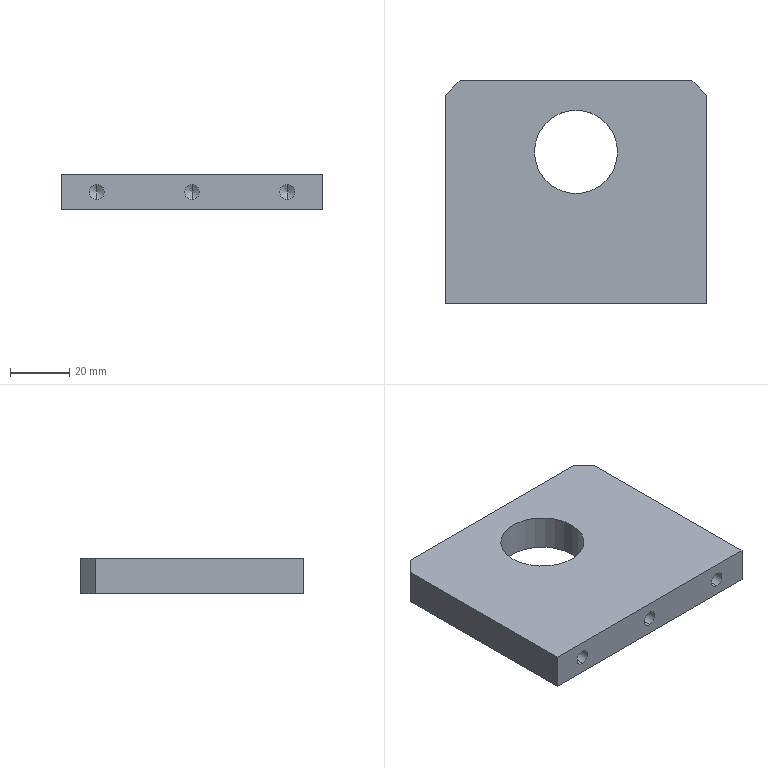Part | STEP file | mounting fixed plate | 1 solid | 22 faces | box 88 x 75 x 12 mm | volume 70480 mm3 | cylinder 8 | plane 8 | cone 6 | commonest cylinder face diameters 5 x6 28 x2
STEP:
#1=CARTESIAN_POINT('',(0.,0.,0.));
#2=DIRECTION('',(0.,0.,1.));
#3=DIRECTION('',(1.,0.,0.));
#4=AXIS2_PLACEMENT_3D('',#1,#2,#3);
#5=CARTESIAN_POINT('',(-14.,13.5,12.));
#6=VERTEX_POINT('',#5);
#7=CARTESIAN_POINT('',(-14.,13.5,0.));
#8=VERTEX_POINT('',#7);
#9=CARTESIAN_POINT('',(-14.,13.5,12.));
#10=DIRECTION('',(0.,0.,-1.));
#11=VECTOR('',#10,1.);
#12=LINE('',#9,#11);
#13=CARTESIAN_POINT('',(0.,13.5,12.));
#14=DIRECTION('',(0.,0.,-1.));
#15=DIRECTION('',(-1.,0.,0.));
#16=AXIS2_PLACEMENT_3D('',#13,#14,#15);
#17=CYLINDRICAL_SURFACE('',#16,14.);
#18=CARTESIAN_POINT('',(6.283,0.));
#19=DIRECTION('',(0.,1.));
#20=VECTOR('',#19,1.);
#21=LINE('',#18,#20);
#22=(GEOMETRIC_REPRESENTATION_CONTEXT(2)PARAMETRIC_REPRESENTATION_CONTEXT()REPRESENTATION_CONTEXT('',''));
#23=DEFINITIONAL_REPRESENTATION('',(#21),#22);
#24=PCURVE('',#17,#23);
#25=CARTESIAN_POINT('',(0.,13.5,12.));
#26=DIRECTION('',(0.,0.,-1.));
#27=DIRECTION('',(-1.,0.,0.));
#28=AXIS2_PLACEMENT_3D('',#25,#26,#27);
#29=CYLINDRICAL_SURFACE('',#28,14.);
#30=CARTESIAN_POINT('',(0.,0.));
#31=DIRECTION('',(0.,1.));
#32=VECTOR('',#31,1.);
#33=LINE('',#30,#32);
#34=(GEOMETRIC_REPRESENTATION_CONTEXT(2)PARAMETRIC_REPRESENTATION_CONTEXT()REPRESENTATION_CONTEXT('',''));
#35=DEFINITIONAL_REPRESENTATION('',(#33),#34);
#36=PCURVE('',#29,#35);
#37=SURFACE_CURVE('',#12,(#24,#36),.PCURVE_S1.);
#38=EDGE_CURVE('',#6,#8,#37,.T.);
#39=ORIENTED_EDGE('',*,*,#38,.T.);
#40=CARTESIAN_POINT('',(14.,13.5,0.));
#41=VERTEX_POINT('',#40);
#42=CARTESIAN_POINT('',(0.,13.5,0.));
#43=DIRECTION('',(0.,0.,1.));
#44=DIRECTION('',(-1.,0.,0.));
#45=AXIS2_PLACEMENT_3D('',#42,#43,#44);
#46=CIRCLE('',#45,14.);
#47=CARTESIAN_POINT('',(6.283,12.));
#48=DIRECTION('',(-1.,0.));
#49=VECTOR('',#48,1.);
#50=LINE('',#47,#49);
#51=(GEOMETRIC_REPRESENTATION_CONTEXT(2)PARAMETRIC_REPRESENTATION_CONTEXT()REPRESENTATION_CONTEXT('',''));
#52=DEFINITIONAL_REPRESENTATION('',(#50),#51);
#53=PCURVE('',#17,#52);
#54=CARTESIAN_POINT('',(-44.,37.5,0.));
#55=DIRECTION('',(0.,0.,-1.));
#56=DIRECTION('',(-1.,0.,0.));
#57=AXIS2_PLACEMENT_3D('',#54,#55,#56);
#58=PLANE('',#57);
#59=CARTESIAN_POINT('',(-30.,-24.));
#60=CARTESIAN_POINT('',(-30.,-48.249));
#61=CARTESIAN_POINT('',(-51.,-36.124));
#62=CARTESIAN_POINT('',(-72.,-24.));
#63=CARTESIAN_POINT('',(-51.,-11.876));
#64=CARTESIAN_POINT('',(-30.,0.2487));
#65=CARTESIAN_POINT('',(-30.,-24.));
#66=(BOUNDED_CURVE()B_SPLINE_CURVE(2,(#59,#60,#61,#62,#63,#64,#65),.UNSPECIFIED.,.T.,.F.)B_SPLINE_CURVE_WITH_KNOTS((1,2,2,2,2,1),(-2.094,0.,2.094,4.189,6.283,8.378),.UNSPECIFIED.)CURVE()GEOMETRIC_REPRESENTATION_ITEM()RATIONAL_B_SPLINE_CURVE((1.,0.5,1.,0.5,1.,0.5,1.))REPRESENTATION_ITEM(''));
#67=(GEOMETRIC_REPRESENTATION_CONTEXT(2)PARAMETRIC_REPRESENTATION_CONTEXT()REPRESENTATION_CONTEXT('',''));
#68=DEFINITIONAL_REPRESENTATION('',(#66),#67);
#69=PCURVE('',#58,#68);
#70=SURFACE_CURVE('',#46,(#53,#69),.PCURVE_S1.);
#71=EDGE_CURVE('',#8,#41,#70,.T.);
#72=ORIENTED_EDGE('',*,*,#71,.T.);
#73=CARTESIAN_POINT('',(14.,13.5,12.));
#74=VERTEX_POINT('',#73);
#75=CARTESIAN_POINT('',(14.,13.5,12.));
#76=DIRECTION('',(0.,0.,-1.));
#77=VECTOR('',#76,1.);
#78=LINE('',#75,#77);
#79=CARTESIAN_POINT('',(3.142,0.));
#80=DIRECTION('',(0.,1.));
#81=VECTOR('',#80,1.);
#82=LINE('',#79,#81);
#83=(GEOMETRIC_REPRESENTATION_CONTEXT(2)PARAMETRIC_REPRESENTATION_CONTEXT()REPRESENTATION_CONTEXT('',''));
#84=DEFINITIONAL_REPRESENTATION('',(#82),#83);
#85=PCURVE('',#17,#84);
#86=CARTESIAN_POINT('',(3.142,0.));
#87=DIRECTION('',(0.,1.));
#88=VECTOR('',#87,1.);
#89=LINE('',#86,#88);
#90=(GEOMETRIC_REPRESENTATION_CONTEXT(2)PARAMETRIC_REPRESENTATION_CONTEXT()REPRESENTATION_CONTEXT('',''));
#91=DEFINITIONAL_REPRESENTATION('',(#89),#90);
#92=PCURVE('',#29,#91);
#93=SURFACE_CURVE('',#78,(#85,#92),.PCURVE_S1.);
#94=EDGE_CURVE('',#74,#41,#93,.T.);
#95=ORIENTED_EDGE('',*,*,#94,.F.);
#96=CARTESIAN_POINT('',(0.,13.5,12.));
#97=DIRECTION('',(0.,0.,1.));
#98=DIRECTION('',(-1.,0.,0.));
#99=AXIS2_PLACEMENT_3D('',#96,#97,#98);
#100=CIRCLE('',#99,14.);
#101=CARTESIAN_POINT('',(6.283,0.));
#102=DIRECTION('',(-1.,0.));
#103=VECTOR('',#102,1.);
#104=LINE('',#101,#103);
#105=(GEOMETRIC_REPRESENTATION_CONTEXT(2)PARAMETRIC_REPRESENTATION_CONTEXT()REPRESENTATION_CONTEXT('',''));
#106=DEFINITIONAL_REPRESENTATION('',(#104),#105);
#107=PCURVE('',#17,#106);
#108=CARTESIAN_POINT('',(-44.,37.5,12.));
#109=DIRECTION('',(0.,0.,-1.));
#110=DIRECTION('',(-1.,0.,0.));
#111=AXIS2_PLACEMENT_3D('',#108,#109,#110);
#112=PLANE('',#111);
#113=CARTESIAN_POINT('',(-30.,-24.));
#114=CARTESIAN_POINT('',(-30.,-48.249));
#115=CARTESIAN_POINT('',(-51.,-36.124));
#116=CARTESIAN_POINT('',(-72.,-24.));
#117=CARTESIAN_POINT('',(-51.,-11.876));
#118=CARTESIAN_POINT('',(-30.,0.2487));
#119=CARTESIAN_POINT('',(-30.,-24.));
#120=(BOUNDED_CURVE()B_SPLINE_CURVE(2,(#113,#114,#115,#116,#117,#118,#119),.UNSPECIFIED.,.T.,.F.)B_SPLINE_CURVE_WITH_KNOTS((1,2,2,2,2,1),(-2.094,0.,2.094,4.189,6.283,8.378),.UNSPECIFIED.)CURVE()GEOMETRIC_REPRESENTATION_ITEM()RATIONAL_B_SPLINE_CURVE((1.,0.5,1.,0.5,1.,0.5,1.))REPRESENTATION_ITEM(''));
#121=(GEOMETRIC_REPRESENTATION_CONTEXT(2)PARAMETRIC_REPRESENTATION_CONTEXT()REPRESENTATION_CONTEXT('',''));
#122=DEFINITIONAL_REPRESENTATION('',(#120),#121);
#123=PCURVE('',#112,#122);
#124=SURFACE_CURVE('',#100,(#107,#123),.PCURVE_S1.);
#125=EDGE_CURVE('',#6,#74,#124,.T.);
#126=ORIENTED_EDGE('',*,*,#125,.F.);
#127=EDGE_LOOP('',(#39,#72,#95,#126));
#128=FACE_BOUND('',#127,.F.);
#129=ADVANCED_FACE('',(#128),#17,.F.);
#130=CARTESIAN_POINT('',(-32.,-20.5,3.5));
#131=VERTEX_POINT('',#130);
#132=CARTESIAN_POINT('',(-32.,-37.5,3.5));
#133=VERTEX_POINT('',#132);
#134=CARTESIAN_POINT('',(-32.,-37.5,3.5));
#135=DIRECTION('',(0.,-1.,0.));
#136=VECTOR('',#135,1.);
#137=LINE('',#134,#136);
#138=CARTESIAN_POINT('',(-32.,-37.5,6.));
#139=DIRECTION('',(0.,-1.,0.));
#140=DIRECTION('',(0.,0.,-1.));
#141=AXIS2_PLACEMENT_3D('',#138,#139,#140);
#142=CYLINDRICAL_SURFACE('',#141,2.5);
#143=CARTESIAN_POINT('',(6.283,0.));
#144=DIRECTION('',(0.,1.));
#145=VECTOR('',#144,1.);
#146=LINE('',#143,#145);
#147=(GEOMETRIC_REPRESENTATION_CONTEXT(2)PARAMETRIC_REPRESENTATION_CONTEXT()REPRESENTATION_CONTEXT('',''));
#148=DEFINITIONAL_REPRESENTATION('',(#146),#147);
#149=PCURVE('',#142,#148);
#150=CARTESIAN_POINT('',(-32.,-37.5,6.));
#151=DIRECTION('',(0.,-1.,0.));
#152=DIRECTION('',(0.,0.,-1.));
#153=AXIS2_PLACEMENT_3D('',#150,#151,#152);
#154=CYLINDRICAL_SURFACE('',#153,2.5);
#155=CARTESIAN_POINT('',(0.,0.));
#156=DIRECTION('',(0.,1.));
#157=VECTOR('',#156,1.);
#158=LINE('',#155,#157);
#159=(GEOMETRIC_REPRESENTATION_CONTEXT(2)PARAMETRIC_REPRESENTATION_CONTEXT()REPRESENTATION_CONTEXT('',''));
#160=DEFINITIONAL_REPRESENTATION('',(#158),#159);
#161=PCURVE('',#154,#160);
#162=SURFACE_CURVE('',#137,(#149,#161),.PCURVE_S1.);
#163=EDGE_CURVE('',#131,#133,#162,.T.);
#164=ORIENTED_EDGE('',*,*,#163,.T.);
#165=CARTESIAN_POINT('',(-32.,-37.5,8.5));
#166=VERTEX_POINT('',#165);
#167=CARTESIAN_POINT('',(-32.,-37.5,6.));
#168=DIRECTION('',(0.,-1.,0.));
#169=DIRECTION('',(0.,0.,-1.));
#170=AXIS2_PLACEMENT_3D('',#167,#168,#169);
#171=CIRCLE('',#170,2.5);
#172=CARTESIAN_POINT('',(0.,0.));
#173=DIRECTION('',(1.,0.));
#174=VECTOR('',#173,1.);
#175=LINE('',#172,#174);
#176=(GEOMETRIC_REPRESENTATION_CONTEXT(2)PARAMETRIC_REPRESENTATION_CONTEXT()REPRESENTATION_CONTEXT('',''));
#177=DEFINITIONAL_REPRESENTATION('',(#175),#176);
#178=PCURVE('',#142,#177);
#179=CARTESIAN_POINT('',(-44.,-37.5,12.));
#180=DIRECTION('',(0.,1.,0.));
#181=DIRECTION('',(0.,0.,1.));
#182=AXIS2_PLACEMENT_3D('',#179,#180,#181);
#183=PLANE('',#182);
#184=CARTESIAN_POINT('',(-8.5,12.));
#185=CARTESIAN_POINT('',(-8.5,16.33));
#186=CARTESIAN_POINT('',(-4.75,14.165));
#187=CARTESIAN_POINT('',(-1.,12.));
#188=CARTESIAN_POINT('',(-4.75,9.835));
#189=CARTESIAN_POINT('',(-8.5,7.67));
#190=CARTESIAN_POINT('',(-8.5,12.));
#191=(BOUNDED_CURVE()B_SPLINE_CURVE(2,(#184,#185,#186,#187,#188,#189,#190),.UNSPECIFIED.,.T.,.F.)B_SPLINE_CURVE_WITH_KNOTS((1,2,2,2,2,1),(-2.094,0.,2.094,4.189,6.283,8.378),.UNSPECIFIED.)CURVE()GEOMETRIC_REPRESENTATION_ITEM()RATIONAL_B_SPLINE_CURVE((1.,0.5,1.,0.5,1.,0.5,1.))REPRESENTATION_ITEM(''));
#192=(GEOMETRIC_REPRESENTATION_CONTEXT(2)PARAMETRIC_REPRESENTATION_CONTEXT()REPRESENTATION_CONTEXT('',''));
#193=DEFINITIONAL_REPRESENTATION('',(#191),#192);
#194=PCURVE('',#183,#193);
#195=SURFACE_CURVE('',#171,(#178,#194),.PCURVE_S1.);
#196=EDGE_CURVE('',#166,#133,#195,.T.);
#197=ORIENTED_EDGE('',*,*,#196,.F.);
#198=CARTESIAN_POINT('',(-32.,-20.5,8.5));
#199=VERTEX_POINT('',#198);
#200=CARTESIAN_POINT('',(-32.,-37.5,8.5));
#201=DIRECTION('',(0.,-1.,0.));
#202=VECTOR('',#201,1.);
#203=LINE('',#200,#202);
#204=CARTESIAN_POINT('',(3.142,0.));
#205=DIRECTION('',(0.,1.));
#206=VECTOR('',#205,1.);
#207=LINE('',#204,#206);
#208=(GEOMETRIC_REPRESENTATION_CONTEXT(2)PARAMETRIC_REPRESENTATION_CONTEXT()REPRESENTATION_CONTEXT('',''));
#209=DEFINITIONAL_REPRESENTATION('',(#207),#208);
#210=PCURVE('',#142,#209);
#211=CARTESIAN_POINT('',(3.142,0.));
#212=DIRECTION('',(0.,1.));
#213=VECTOR('',#212,1.);
#214=LINE('',#211,#213);
#215=(GEOMETRIC_REPRESENTATION_CONTEXT(2)PARAMETRIC_REPRESENTATION_CONTEXT()REPRESENTATION_CONTEXT('',''));
#216=DEFINITIONAL_REPRESENTATION('',(#214),#215);
#217=PCURVE('',#154,#216);
#218=SURFACE_CURVE('',#203,(#210,#217),.PCURVE_S1.);
#219=EDGE_CURVE('',#199,#166,#218,.T.);
#220=ORIENTED_EDGE('',*,*,#219,.F.);
#221=CARTESIAN_POINT('',(-32.,-20.5,6.));
#222=DIRECTION('',(0.,-1.,0.));
#223=DIRECTION('',(0.,0.,-1.));
#224=AXIS2_PLACEMENT_3D('',#221,#222,#223);
#225=CIRCLE('',#224,2.5);
#226=CARTESIAN_POINT('',(0.,-17.));
#227=DIRECTION('',(1.,0.));
#228=VECTOR('',#227,1.);
#229=LINE('',#226,#228);
#230=(GEOMETRIC_REPRESENTATION_CONTEXT(2)PARAMETRIC_REPRESENTATION_CONTEXT()REPRESENTATION_CONTEXT('',''));
#231=DEFINITIONAL_REPRESENTATION('',(#229),#230);
#232=PCURVE('',#142,#231);
#233=CARTESIAN_POINT('',(-32.,-20.5,6.));
#234=DIRECTION('',(0.,-1.,0.));
#235=DIRECTION('',(0.,0.,-1.));
#236=AXIS2_PLACEMENT_3D('',#233,#234,#235);
#237=CONICAL_SURFACE('',#236,2.5,1.03);
#238=CARTESIAN_POINT('',(0.,0.));
#239=DIRECTION('',(1.,0.));
#240=VECTOR('',#239,1.);
#241=LINE('',#238,#240);
#242=(GEOMETRIC_REPRESENTATION_CONTEXT(2)PARAMETRIC_REPRESENTATION_CONTEXT()REPRESENTATION_CONTEXT('',''));
#243=DEFINITIONAL_REPRESENTATION('',(#241),#242);
#244=PCURVE('',#237,#243);
#245=SURFACE_CURVE('',#225,(#232,#244),.PCURVE_S1.);
#246=EDGE_CURVE('',#199,#131,#245,.T.);
#247=ORIENTED_EDGE('',*,*,#246,.T.);
#248=EDGE_LOOP('',(#164,#197,#220,#247));
#249=FACE_BOUND('',#248,.F.);
#250=ADVANCED_FACE('',(#249),#142,.F.);
#251=CARTESIAN_POINT('',(32.,-20.5,3.5));
#252=VERTEX_POINT('',#251);
#253=CARTESIAN_POINT('',(32.,-37.5,3.5));
#254=VERTEX_POINT('',#253);
#255=CARTESIAN_POINT('',(32.,-37.5,3.5));
#256=DIRECTION('',(0.,-1.,0.));
#257=VECTOR('',#256,1.);
#258=LINE('',#255,#257);
#259=CARTESIAN_POINT('',(32.,-37.5,6.));
#260=DIRECTION('',(0.,-1.,0.));
#261=DIRECTION('',(0.,0.,-1.));
#262=AXIS2_PLACEMENT_3D('',#259,#260,#261);
#263=CYLINDRICAL_SURFACE('',#262,2.5);
#264=CARTESIAN_POINT('',(6.283,0.));
#265=DIRECTION('',(0.,1.));
#266=VECTOR('',#265,1.);
#267=LINE('',#264,#266);
#268=(GEOMETRIC_REPRESENTATION_CONTEXT(2)PARAMETRIC_REPRESENTATION_CONTEXT()REPRESENTATION_CONTEXT('',''));
#269=DEFINITIONAL_REPRESENTATION('',(#267),#268);
#270=PCURVE('',#263,#269);
#271=CARTESIAN_POINT('',(32.,-37.5,6.));
#272=DIRECTION('',(0.,-1.,0.));
#273=DIRECTION('',(0.,0.,-1.));
#274=AXIS2_PLACEMENT_3D('',#271,#272,#273);
#275=CYLINDRICAL_SURFACE('',#274,2.5);
#276=CARTESIAN_POINT('',(0.,0.));
#277=DIRECTION('',(0.,1.));
#278=VECTOR('',#277,1.);
#279=LINE('',#276,#278);
#280=(GEOMETRIC_REPRESENTATION_CONTEXT(2)PARAMETRIC_REPRESENTATION_CONTEXT()REPRESENTATION_CONTEXT('',''));
#281=DEFINITIONAL_REPRESENTATION('',(#279),#280);
#282=PCURVE('',#275,#281);
#283=SURFACE_CURVE('',#258,(#270,#282),.PCURVE_S1.);
#284=EDGE_CURVE('',#252,#254,#283,.T.);
#285=ORIENTED_EDGE('',*,*,#284,.T.);
#286=CARTESIAN_POINT('',(32.,-37.5,8.5));
#287=VERTEX_POINT('',#286);
#288=CARTESIAN_POINT('',(32.,-37.5,6.));
#289=DIRECTION('',(0.,-1.,0.));
#290=DIRECTION('',(0.,0.,-1.));
#291=AXIS2_PLACEMENT_3D('',#288,#289,#290);
#292=CIRCLE('',#291,2.5);
#293=CARTESIAN_POINT('',(0.,0.));
#294=DIRECTION('',(1.,0.));
#295=VECTOR('',#294,1.);
#296=LINE('',#293,#295);
#297=(GEOMETRIC_REPRESENTATION_CONTEXT(2)PARAMETRIC_REPRESENTATION_CONTEXT()REPRESENTATION_CONTEXT('',''));
#298=DEFINITIONAL_REPRESENTATION('',(#296),#297);
#299=PCURVE('',#263,#298);
#300=CARTESIAN_POINT('',(-8.5,76.));
#301=CARTESIAN_POINT('',(-8.5,80.33));
#302=CARTESIAN_POINT('',(-4.75,78.165));
#303=CARTESIAN_POINT('',(-1.,76.));
#304=CARTESIAN_POINT('',(-4.75,73.835));
#305=CARTESIAN_POINT('',(-8.5,71.67));
#306=CARTESIAN_POINT('',(-8.5,76.));
#307=(BOUNDED_CURVE()B_SPLINE_CURVE(2,(#300,#301,#302,#303,#304,#305,#306),.UNSPECIFIED.,.T.,.F.)B_SPLINE_CURVE_WITH_KNOTS((1,2,2,2,2,1),(-2.094,0.,2.094,4.189,6.283,8.378),.UNSPECIFIED.)CURVE()GEOMETRIC_REPRESENTATION_ITEM()RATIONAL_B_SPLINE_CURVE((1.,0.5,1.,0.5,1.,0.5,1.))REPRESENTATION_ITEM(''));
#308=(GEOMETRIC_REPRESENTATION_CONTEXT(2)PARAMETRIC_REPRESENTATION_CONTEXT()REPRESENTATION_CONTEXT('',''));
#309=DEFINITIONAL_REPRESENTATION('',(#307),#308);
#310=PCURVE('',#183,#309);
#311=SURFACE_CURVE('',#292,(#299,#310),.PCURVE_S1.);
#312=EDGE_CURVE('',#287,#254,#311,.T.);
#313=ORIENTED_EDGE('',*,*,#312,.F.);
#314=CARTESIAN_POINT('',(32.,-20.5,8.5));
#315=VERTEX_POINT('',#314);
#316=CARTESIAN_POINT('',(32.,-37.5,8.5));
#317=DIRECTION('',(0.,-1.,0.));
#318=VECTOR('',#317,1.);
#319=LINE('',#316,#318);
#320=CARTESIAN_POINT('',(3.142,0.));
#321=DIRECTION('',(0.,1.));
#322=VECTOR('',#321,1.);
#323=LINE('',#320,#322);
#324=(GEOMETRIC_REPRESENTATION_CONTEXT(2)PARAMETRIC_REPRESENTATION_CONTEXT()REPRESENTATION_CONTEXT('',''));
#325=DEFINITIONAL_REPRESENTATION('',(#323),#324);
#326=PCURVE('',#263,#325);
#327=CARTESIAN_POINT('',(3.142,0.));
#328=DIRECTION('',(0.,1.));
#329=VECTOR('',#328,1.);
#330=LINE('',#327,#329);
#331=(GEOMETRIC_REPRESENTATION_CONTEXT(2)PARAMETRIC_REPRESENTATION_CONTEXT()REPRESENTATION_CONTEXT('',''));
#332=DEFINITIONAL_REPRESENTATION('',(#330),#331);
#333=PCURVE('',#275,#332);
#334=SURFACE_CURVE('',#319,(#326,#333),.PCURVE_S1.);
#335=EDGE_CURVE('',#315,#287,#334,.T.);
#336=ORIENTED_EDGE('',*,*,#335,.F.);
#337=CARTESIAN_POINT('',(32.,-20.5,6.));
#338=DIRECTION('',(0.,-1.,0.));
#339=DIRECTION('',(0.,0.,-1.));
#340=AXIS2_PLACEMENT_3D('',#337,#338,#339);
#341=CIRCLE('',#340,2.5);
#342=CARTESIAN_POINT('',(0.,-17.));
#343=DIRECTION('',(1.,0.));
#344=VECTOR('',#343,1.);
#345=LINE('',#342,#344);
#346=(GEOMETRIC_REPRESENTATION_CONTEXT(2)PARAMETRIC_REPRESENTATION_CONTEXT()REPRESENTATION_CONTEXT('',''));
#347=DEFINITIONAL_REPRESENTATION('',(#345),#346);
#348=PCURVE('',#263,#347);
#349=CARTESIAN_POINT('',(32.,-20.5,6.));
#350=DIRECTION('',(0.,-1.,0.));
#351=DIRECTION('',(0.,0.,-1.));
#352=AXIS2_PLACEMENT_3D('',#349,#350,#351);
#353=CONICAL_SURFACE('',#352,2.5,1.03);
#354=CARTESIAN_POINT('',(0.,0.));
#355=DIRECTION('',(1.,0.));
#356=VECTOR('',#355,1.);
#357=LINE('',#354,#356);
#358=(GEOMETRIC_REPRESENTATION_CONTEXT(2)PARAMETRIC_REPRESENTATION_CONTEXT()REPRESENTATION_CONTEXT('',''));
#359=DEFINITIONAL_REPRESENTATION('',(#357),#358);
#360=PCURVE('',#353,#359);
#361=SURFACE_CURVE('',#341,(#348,#360),.PCURVE_S1.);
#362=EDGE_CURVE('',#315,#252,#361,.T.);
#363=ORIENTED_EDGE('',*,*,#362,.T.);
#364=EDGE_LOOP('',(#285,#313,#336,#363));
#365=FACE_BOUND('',#364,.F.);
#366=ADVANCED_FACE('',(#365),#263,.F.);
#367=CARTESIAN_POINT('',(0.,-20.5,3.5));
#368=VERTEX_POINT('',#367);
#369=CARTESIAN_POINT('',(0.,-37.5,3.5));
#370=VERTEX_POINT('',#369);
#371=CARTESIAN_POINT('',(0.,-37.5,3.5));
#372=DIRECTION('',(0.,-1.,0.));
#373=VECTOR('',#372,1.);
#374=LINE('',#371,#373);
#375=CARTESIAN_POINT('',(0.,-37.5,6.));
#376=DIRECTION('',(0.,-1.,0.));
#377=DIRECTION('',(0.,0.,-1.));
#378=AXIS2_PLACEMENT_3D('',#375,#376,#377);
#379=CYLINDRICAL_SURFACE('',#378,2.5);
#380=CARTESIAN_POINT('',(6.283,0.));
#381=DIRECTION('',(0.,1.));
#382=VECTOR('',#381,1.);
#383=LINE('',#380,#382);
#384=(GEOMETRIC_REPRESENTATION_CONTEXT(2)PARAMETRIC_REPRESENTATION_CONTEXT()REPRESENTATION_CONTEXT('',''));
#385=DEFINITIONAL_REPRESENTATION('',(#383),#384);
#386=PCURVE('',#379,#385);
#387=CARTESIAN_POINT('',(0.,-37.5,6.));
#388=DIRECTION('',(0.,-1.,0.));
#389=DIRECTION('',(0.,0.,-1.));
#390=AXIS2_PLACEMENT_3D('',#387,#388,#389);
#391=CYLINDRICAL_SURFACE('',#390,2.5);
#392=CARTESIAN_POINT('',(0.,0.));
#393=DIRECTION('',(0.,1.));
#394=VECTOR('',#393,1.);
#395=LINE('',#392,#394);
#396=(GEOMETRIC_REPRESENTATION_CONTEXT(2)PARAMETRIC_REPRESENTATION_CONTEXT()REPRESENTATION_CONTEXT('',''));
#397=DEFINITIONAL_REPRESENTATION('',(#395),#396);
#398=PCURVE('',#391,#397);
#399=SURFACE_CURVE('',#374,(#386,#398),.PCURVE_S1.);
#400=EDGE_CURVE('',#368,#370,#399,.T.);
#401=ORIENTED_EDGE('',*,*,#400,.T.);
#402=CARTESIAN_POINT('',(0.,-37.5,8.5));
#403=VERTEX_POINT('',#402);
#404=CARTESIAN_POINT('',(0.,-37.5,6.));
#405=DIRECTION('',(0.,-1.,0.));
#406=DIRECTION('',(0.,0.,-1.));
#407=AXIS2_PLACEMENT_3D('',#404,#405,#406);
#408=CIRCLE('',#407,2.5);
#409=CARTESIAN_POINT('',(0.,0.));
#410=DIRECTION('',(1.,0.));
#411=VECTOR('',#410,1.);
#412=LINE('',#409,#411);
#413=(GEOMETRIC_REPRESENTATION_CONTEXT(2)PARAMETRIC_REPRESENTATION_CONTEXT()REPRESENTATION_CONTEXT('',''));
#414=DEFINITIONAL_REPRESENTATION('',(#412),#413);
#415=PCURVE('',#379,#414);
#416=CARTESIAN_POINT('',(-8.5,44.));
#417=CARTESIAN_POINT('',(-8.5,48.33));
#418=CARTESIAN_POINT('',(-4.75,46.165));
#419=CARTESIAN_POINT('',(-1.,44.));
#420=CARTESIAN_POINT('',(-4.75,41.835));
#421=CARTESIAN_POINT('',(-8.5,39.67));
#422=CARTESIAN_POINT('',(-8.5,44.));
#423=(BOUNDED_CURVE()B_SPLINE_CURVE(2,(#416,#417,#418,#419,#420,#421,#422),.UNSPECIFIED.,.T.,.F.)B_SPLINE_CURVE_WITH_KNOTS((1,2,2,2,2,1),(-2.094,0.,2.094,4.189,6.283,8.378),.UNSPECIFIED.)CURVE()GEOMETRIC_REPRESENTATION_ITEM()RATIONAL_B_SPLINE_CURVE((1.,0.5,1.,0.5,1.,0.5,1.))REPRESENTATION_ITEM(''));
#424=(GEOMETRIC_REPRESENTATION_CONTEXT(2)PARAMETRIC_REPRESENTATION_CONTEXT()REPRESENTATION_CONTEXT('',''));
#425=DEFINITIONAL_REPRESENTATION('',(#423),#424);
#426=PCURVE('',#183,#425);
#427=SURFACE_CURVE('',#408,(#415,#426),.PCURVE_S1.);
#428=EDGE_CURVE('',#403,#370,#427,.T.);
#429=ORIENTED_EDGE('',*,*,#428,.F.);
#430=CARTESIAN_POINT('',(0.,-20.5,8.5));
#431=VERTEX_POINT('',#430);
#432=CARTESIAN_POINT('',(0.,-37.5,8.5));
#433=DIRECTION('',(0.,-1.,0.));
#434=VECTOR('',#433,1.);
#435=LINE('',#432,#434);
#436=CARTESIAN_POINT('',(3.142,0.));
#437=DIRECTION('',(0.,1.));
#438=VECTOR('',#437,1.);
#439=LINE('',#436,#438);
#440=(GEOMETRIC_REPRESENTATION_CONTEXT(2)PARAMETRIC_REPRESENTATION_CONTEXT()REPRESENTATION_CONTEXT('',''));
#441=DEFINITIONAL_REPRESENTATION('',(#439),#440);
#442=PCURVE('',#379,#441);
#443=CARTESIAN_POINT('',(3.142,0.));
#444=DIRECTION('',(0.,1.));
#445=VECTOR('',#444,1.);
#446=LINE('',#443,#445);
#447=(GEOMETRIC_REPRESENTATION_CONTEXT(2)PARAMETRIC_REPRESENTATION_CONTEXT()REPRESENTATION_CONTEXT('',''));
#448=DEFINITIONAL_REPRESENTATION('',(#446),#447);
#449=PCURVE('',#391,#448);
#450=SURFACE_CURVE('',#435,(#442,#449),.PCURVE_S1.);
#451=EDGE_CURVE('',#431,#403,#450,.T.);
#452=ORIENTED_EDGE('',*,*,#451,.F.);
#453=CARTESIAN_POINT('',(0.,-20.5,6.));
#454=DIRECTION('',(0.,-1.,0.));
#455=DIRECTION('',(0.,0.,-1.));
#456=AXIS2_PLACEMENT_3D('',#453,#454,#455);
#457=CIRCLE('',#456,2.5);
#458=CARTESIAN_POINT('',(0.,-17.));
#459=DIRECTION('',(1.,0.));
#460=VECTOR('',#459,1.);
#461=LINE('',#458,#460);
#462=(GEOMETRIC_REPRESENTATION_CONTEXT(2)PARAMETRIC_REPRESENTATION_CONTEXT()REPRESENTATION_CONTEXT('',''));
#463=DEFINITIONAL_REPRESENTATION('',(#461),#462);
#464=PCURVE('',#379,#463);
#465=CARTESIAN_POINT('',(0.,-20.5,6.));
#466=DIRECTION('',(0.,-1.,0.));
#467=DIRECTION('',(0.,0.,-1.));
#468=AXIS2_PLACEMENT_3D('',#465,#466,#467);
#469=CONICAL_SURFACE('',#468,2.5,1.03);
#470=CARTESIAN_POINT('',(0.,0.));
#471=DIRECTION('',(1.,0.));
#472=VECTOR('',#471,1.);
#473=LINE('',#470,#472);
#474=(GEOMETRIC_REPRESENTATION_CONTEXT(2)PARAMETRIC_REPRESENTATION_CONTEXT()REPRESENTATION_CONTEXT('',''));
#475=DEFINITIONAL_REPRESENTATION('',(#473),#474);
#476=PCURVE('',#469,#475);
#477=SURFACE_CURVE('',#457,(#464,#476),.PCURVE_S1.);
#478=EDGE_CURVE('',#431,#368,#477,.T.);
#479=ORIENTED_EDGE('',*,*,#478,.T.);
#480=EDGE_LOOP('',(#401,#429,#452,#479));
#481=FACE_BOUND('',#480,.F.);
#482=ADVANCED_FACE('',(#481),#379,.F.);
#483=ORIENTED_EDGE('',*,*,#246,.F.);
#484=CARTESIAN_POINT('',(-32.,-18.998,6.));
#485=VERTEX_POINT('',#484);
#486=CARTESIAN_POINT('',(-32.,-20.5,8.5));
#487=DIRECTION('',(0.,-0.515,0.8572));
#488=VECTOR('',#487,1.);
#489=LINE('',#486,#488);
#490=CARTESIAN_POINT('',(3.142,0.));
#491=DIRECTION('',(0.,1.));
#492=VECTOR('',#491,1.);
#493=LINE('',#490,#492);
#494=(GEOMETRIC_REPRESENTATION_CONTEXT(2)PARAMETRIC_REPRESENTATION_CONTEXT()REPRESENTATION_CONTEXT('',''));
#495=DEFINITIONAL_REPRESENTATION('',(#493),#494);
#496=PCURVE('',#237,#495);
#497=CARTESIAN_POINT('',(-32.,-20.5,6.));
#498=DIRECTION('',(0.,-1.,0.));
#499=DIRECTION('',(0.,0.,-1.));
#500=AXIS2_PLACEMENT_3D('',#497,#498,#499);
#501=CONICAL_SURFACE('',#500,2.5,1.03);
#502=CARTESIAN_POINT('',(3.142,0.));
#503=DIRECTION('',(0.,1.));
#504=VECTOR('',#503,1.);
#505=LINE('',#502,#504);
#506=(GEOMETRIC_REPRESENTATION_CONTEXT(2)PARAMETRIC_REPRESENTATION_CONTEXT()REPRESENTATION_CONTEXT('',''));
#507=DEFINITIONAL_REPRESENTATION('',(#505),#506);
#508=PCURVE('',#501,#507);
#509=SURFACE_CURVE('',#489,(#496,#508),.PCURVE_S1.);
#510=EDGE_CURVE('',#485,#199,#509,.T.);
#511=ORIENTED_EDGE('',*,*,#510,.F.);
#512=CARTESIAN_POINT('',(-32.,-20.5,3.5));
#513=DIRECTION('',(0.,-0.515,-0.8572));
#514=VECTOR('',#513,1.);
#515=LINE('',#512,#514);
#516=CARTESIAN_POINT('',(6.283,0.));
#517=DIRECTION('',(0.,1.));
#518=VECTOR('',#517,1.);
#519=LINE('',#516,#518);
#520=(GEOMETRIC_REPRESENTATION_CONTEXT(2)PARAMETRIC_REPRESENTATION_CONTEXT()REPRESENTATION_CONTEXT('',''));
#521=DEFINITIONAL_REPRESENTATION('',(#519),#520);
#522=PCURVE('',#237,#521);
#523=CARTESIAN_POINT('',(0.,0.));
#524=DIRECTION('',(0.,1.));
#525=VECTOR('',#524,1.);
#526=LINE('',#523,#525);
#527=(GEOMETRIC_REPRESENTATION_CONTEXT(2)PARAMETRIC_REPRESENTATION_CONTEXT()REPRESENTATION_CONTEXT('',''));
#528=DEFINITIONAL_REPRESENTATION('',(#526),#527);
#529=PCURVE('',#501,#528);
#530=SURFACE_CURVE('',#515,(#522,#529),.PCURVE_S1.);
#531=EDGE_CURVE('',#485,#131,#530,.T.);
#532=ORIENTED_EDGE('',*,*,#531,.T.);
#533=EDGE_LOOP('',(#483,#511,#532));
#534=FACE_BOUND('',#533,.F.);
#535=ADVANCED_FACE('',(#534),#237,.F.);
#536=ORIENTED_EDGE('',*,*,#362,.F.);
#537=CARTESIAN_POINT('',(32.,-18.998,6.));
#538=VERTEX_POINT('',#537);
#539=CARTESIAN_POINT('',(32.,-20.5,8.5));
#540=DIRECTION('',(0.,-0.515,0.8572));
#541=VECTOR('',#540,1.);
#542=LINE('',#539,#541);
#543=CARTESIAN_POINT('',(3.142,0.));
#544=DIRECTION('',(0.,1.));
#545=VECTOR('',#544,1.);
#546=LINE('',#543,#545);
#547=(GEOMETRIC_REPRESENTATION_CONTEXT(2)PARAMETRIC_REPRESENTATION_CONTEXT()REPRESENTATION_CONTEXT('',''));
#548=DEFINITIONAL_REPRESENTATION('',(#546),#547);
#549=PCURVE('',#353,#548);
#550=CARTESIAN_POINT('',(32.,-20.5,6.));
#551=DIRECTION('',(0.,-1.,0.));
#552=DIRECTION('',(0.,0.,-1.));
#553=AXIS2_PLACEMENT_3D('',#550,#551,#552);
#554=CONICAL_SURFACE('',#553,2.5,1.03);
#555=CARTESIAN_POINT('',(3.142,0.));
#556=DIRECTION('',(0.,1.));
#557=VECTOR('',#556,1.);
#558=LINE('',#555,#557);
#559=(GEOMETRIC_REPRESENTATION_CONTEXT(2)PARAMETRIC_REPRESENTATION_CONTEXT()REPRESENTATION_CONTEXT('',''));
#560=DEFINITIONAL_REPRESENTATION('',(#558),#559);
#561=PCURVE('',#554,#560);
#562=SURFACE_CURVE('',#542,(#549,#561),.PCURVE_S1.);
#563=EDGE_CURVE('',#538,#315,#562,.T.);
#564=ORIENTED_EDGE('',*,*,#563,.F.);
#565=CARTESIAN_POINT('',(32.,-20.5,3.5));
#566=DIRECTION('',(0.,-0.515,-0.8572));
#567=VECTOR('',#566,1.);
#568=LINE('',#565,#567);
#569=CARTESIAN_POINT('',(6.283,0.));
#570=DIRECTION('',(0.,1.));
#571=VECTOR('',#570,1.);
#572=LINE('',#569,#571);
#573=(GEOMETRIC_REPRESENTATION_CONTEXT(2)PARAMETRIC_REPRESENTATION_CONTEXT()REPRESENTATION_CONTEXT('',''));
#574=DEFINITIONAL_REPRESENTATION('',(#572),#573);
#575=PCURVE('',#353,#574);
#576=CARTESIAN_POINT('',(0.,0.));
#577=DIRECTION('',(0.,1.));
#578=VECTOR('',#577,1.);
#579=LINE('',#576,#578);
#580=(GEOMETRIC_REPRESENTATION_CONTEXT(2)PARAMETRIC_REPRESENTATION_CONTEXT()REPRESENTATION_CONTEXT('',''));
#581=DEFINITIONAL_REPRESENTATION('',(#579),#580);
#582=PCURVE('',#554,#581);
#583=SURFACE_CURVE('',#568,(#575,#582),.PCURVE_S1.);
#584=EDGE_CURVE('',#538,#252,#583,.T.);
#585=ORIENTED_EDGE('',*,*,#584,.T.);
#586=EDGE_LOOP('',(#536,#564,#585));
#587=FACE_BOUND('',#586,.F.);
#588=ADVANCED_FACE('',(#587),#353,.F.);
#589=ORIENTED_EDGE('',*,*,#478,.F.);
#590=CARTESIAN_POINT('',(0.,-18.998,6.));
#591=VERTEX_POINT('',#590);
#592=CARTESIAN_POINT('',(0.,-20.5,8.5));
#593=DIRECTION('',(0.,-0.515,0.8572));
#594=VECTOR('',#593,1.);
#595=LINE('',#592,#594);
#596=CARTESIAN_POINT('',(3.142,0.));
#597=DIRECTION('',(0.,1.));
#598=VECTOR('',#597,1.);
#599=LINE('',#596,#598);
#600=(GEOMETRIC_REPRESENTATION_CONTEXT(2)PARAMETRIC_REPRESENTATION_CONTEXT()REPRESENTATION_CONTEXT('',''));
#601=DEFINITIONAL_REPRESENTATION('',(#599),#600);
#602=PCURVE('',#469,#601);
#603=CARTESIAN_POINT('',(0.,-20.5,6.));
#604=DIRECTION('',(0.,-1.,0.));
#605=DIRECTION('',(0.,0.,-1.));
#606=AXIS2_PLACEMENT_3D('',#603,#604,#605);
#607=CONICAL_SURFACE('',#606,2.5,1.03);
#608=CARTESIAN_POINT('',(3.142,0.));
#609=DIRECTION('',(0.,1.));
#610=VECTOR('',#609,1.);
#611=LINE('',#608,#610);
#612=(GEOMETRIC_REPRESENTATION_CONTEXT(2)PARAMETRIC_REPRESENTATION_CONTEXT()REPRESENTATION_CONTEXT('',''));
#613=DEFINITIONAL_REPRESENTATION('',(#611),#612);
#614=PCURVE('',#607,#613);
#615=SURFACE_CURVE('',#595,(#602,#614),.PCURVE_S1.);
#616=EDGE_CURVE('',#591,#431,#615,.T.);
#617=ORIENTED_EDGE('',*,*,#616,.F.);
#618=CARTESIAN_POINT('',(0.,-20.5,3.5));
#619=DIRECTION('',(0.,-0.515,-0.8572));
#620=VECTOR('',#619,1.);
#621=LINE('',#618,#620);
#622=CARTESIAN_POINT('',(6.283,0.));
#623=DIRECTION('',(0.,1.));
#624=VECTOR('',#623,1.);
#625=LINE('',#622,#624);
#626=(GEOMETRIC_REPRESENTATION_CONTEXT(2)PARAMETRIC_REPRESENTATION_CONTEXT()REPRESENTATION_CONTEXT('',''));
#627=DEFINITIONAL_REPRESENTATION('',(#625),#626);
#628=PCURVE('',#469,#627);
#629=CARTESIAN_POINT('',(0.,0.));
#630=DIRECTION('',(0.,1.));
#631=VECTOR('',#630,1.);
#632=LINE('',#629,#631);
#633=(GEOMETRIC_REPRESENTATION_CONTEXT(2)PARAMETRIC_REPRESENTATION_CONTEXT()REPRESENTATION_CONTEXT('',''));
#634=DEFINITIONAL_REPRESENTATION('',(#632),#633);
#635=PCURVE('',#607,#634);
#636=SURFACE_CURVE('',#621,(#628,#635),.PCURVE_S1.);
#637=EDGE_CURVE('',#591,#368,#636,.T.);
#638=ORIENTED_EDGE('',*,*,#637,.T.);
#639=EDGE_LOOP('',(#589,#617,#638));
#640=FACE_BOUND('',#639,.F.);
#641=ADVANCED_FACE('',(#640),#469,.F.);
#642=CARTESIAN_POINT('',(-44.,-37.5,12.));
#643=VERTEX_POINT('',#642);
#644=CARTESIAN_POINT('',(-44.,32.5,12.));
#645=VERTEX_POINT('',#644);
#646=CARTESIAN_POINT('',(-44.,37.5,12.));
#647=DIRECTION('',(0.,1.,0.));
#648=VECTOR('',#647,1.);
#649=LINE('',#646,#648);
#650=CARTESIAN_POINT('',(0.,0.));
#651=DIRECTION('',(0.,1.));
#652=VECTOR('',#651,1.);
#653=LINE('',#650,#652);
#654=(GEOMETRIC_REPRESENTATION_CONTEXT(2)PARAMETRIC_REPRESENTATION_CONTEXT()REPRESENTATION_CONTEXT('',''));
#655=DEFINITIONAL_REPRESENTATION('',(#653),#654);
#656=PCURVE('',#112,#655);
#657=CARTESIAN_POINT('',(-44.,-37.5,12.));
#658=DIRECTION('',(1.,0.,0.));
#659=DIRECTION('',(0.,0.,-1.));
#660=AXIS2_PLACEMENT_3D('',#657,#658,#659);
#661=PLANE('',#660);
#662=CARTESIAN_POINT('',(0.,75.));
#663=DIRECTION('',(0.,1.));
#664=VECTOR('',#663,1.);
#665=LINE('',#662,#664);
#666=(GEOMETRIC_REPRESENTATION_CONTEXT(2)PARAMETRIC_REPRESENTATION_CONTEXT()REPRESENTATION_CONTEXT('',''));
#667=DEFINITIONAL_REPRESENTATION('',(#665),#666);
#668=PCURVE('',#661,#667);
#669=SURFACE_CURVE('',#649,(#656,#668),.PCURVE_S1.);
#670=EDGE_CURVE('',#643,#645,#669,.T.);
#671=ORIENTED_EDGE('',*,*,#670,.F.);
#672=CARTESIAN_POINT('',(44.,-37.5,12.));
#673=VERTEX_POINT('',#672);
#674=CARTESIAN_POINT('',(-44.,-37.5,12.));
#675=DIRECTION('',(-1.,0.,0.));
#676=VECTOR('',#675,1.);
#677=LINE('',#674,#676);
#678=CARTESIAN_POINT('',(0.,-75.));
#679=DIRECTION('',(1.,0.));
#680=VECTOR('',#679,1.);
#681=LINE('',#678,#680);
#682=(GEOMETRIC_REPRESENTATION_CONTEXT(2)PARAMETRIC_REPRESENTATION_CONTEXT()REPRESENTATION_CONTEXT('',''));
#683=DEFINITIONAL_REPRESENTATION('',(#681),#682);
#684=PCURVE('',#112,#683);
#685=CARTESIAN_POINT('',(0.,0.));
#686=DIRECTION('',(0.,-1.));
#687=VECTOR('',#686,1.);
#688=LINE('',#685,#687);
#689=(GEOMETRIC_REPRESENTATION_CONTEXT(2)PARAMETRIC_REPRESENTATION_CONTEXT()REPRESENTATION_CONTEXT('',''));
#690=DEFINITIONAL_REPRESENTATION('',(#688),#689);
#691=PCURVE('',#183,#690);
#692=SURFACE_CURVE('',#677,(#684,#691),.PCURVE_S1.);
#693=EDGE_CURVE('',#673,#643,#692,.T.);
#694=ORIENTED_EDGE('',*,*,#693,.F.);
#695=CARTESIAN_POINT('',(44.,32.5,12.));
#696=VERTEX_POINT('',#695);
#697=CARTESIAN_POINT('',(44.,37.5,12.));
#698=DIRECTION('',(0.,-1.,0.));
#699=VECTOR('',#698,1.);
#700=LINE('',#697,#699);
#701=CARTESIAN_POINT('',(-88.,0.));
#702=DIRECTION('',(0.,-1.));
#703=VECTOR('',#702,1.);
#704=LINE('',#701,#703);
#705=(GEOMETRIC_REPRESENTATION_CONTEXT(2)PARAMETRIC_REPRESENTATION_CONTEXT()REPRESENTATION_CONTEXT('',''));
#706=DEFINITIONAL_REPRESENTATION('',(#704),#705);
#707=PCURVE('',#112,#706);
#708=CARTESIAN_POINT('',(44.,-37.5,12.));
#709=DIRECTION('',(-1.,0.,0.));
#710=DIRECTION('',(0.,-1.,0.));
#711=AXIS2_PLACEMENT_3D('',#708,#709,#710);
#712=PLANE('',#711);
#713=CARTESIAN_POINT('',(-75.,0.));
#714=DIRECTION('',(1.,0.));
#715=VECTOR('',#714,1.);
#716=LINE('',#713,#715);
#717=(GEOMETRIC_REPRESENTATION_CONTEXT(2)PARAMETRIC_REPRESENTATION_CONTEXT()REPRESENTATION_CONTEXT('',''));
#718=DEFINITIONAL_REPRESENTATION('',(#716),#717);
#719=PCURVE('',#712,#718);
#720=SURFACE_CURVE('',#700,(#707,#719),.PCURVE_S1.);
#721=EDGE_CURVE('',#696,#673,#720,.T.);
#722=ORIENTED_EDGE('',*,*,#721,.F.);
#723=CARTESIAN_POINT('',(39.,37.5,12.));
#724=VERTEX_POINT('',#723);
#725=CARTESIAN_POINT('',(39.,37.5,12.));
#726=DIRECTION('',(0.7071,-0.7071,0.));
#727=VECTOR('',#726,1.);
#728=LINE('',#725,#727);
#729=CARTESIAN_POINT('',(-83.,0.));
#730=DIRECTION('',(-0.7071,-0.7071));
#731=VECTOR('',#730,1.);
#732=LINE('',#729,#731);
#733=(GEOMETRIC_REPRESENTATION_CONTEXT(2)PARAMETRIC_REPRESENTATION_CONTEXT()REPRESENTATION_CONTEXT('',''));
#734=DEFINITIONAL_REPRESENTATION('',(#732),#733);
#735=PCURVE('',#112,#734);
#736=CARTESIAN_POINT('',(39.,37.5,12.));
#737=DIRECTION('',(-0.7071,-0.7071,0.));
#738=DIRECTION('',(0.7071,-0.7071,0.));
#739=AXIS2_PLACEMENT_3D('',#736,#737,#738);
#740=PLANE('',#739);
#741=CARTESIAN_POINT('',(0.,0.));
#742=DIRECTION('',(1.,0.));
#743=VECTOR('',#742,1.);
#744=LINE('',#741,#743);
#745=(GEOMETRIC_REPRESENTATION_CONTEXT(2)PARAMETRIC_REPRESENTATION_CONTEXT()REPRESENTATION_CONTEXT('',''));
#746=DEFINITIONAL_REPRESENTATION('',(#744),#745);
#747=PCURVE('',#740,#746);
#748=SURFACE_CURVE('',#728,(#735,#747),.PCURVE_S1.);
#749=EDGE_CURVE('',#724,#696,#748,.T.);
#750=ORIENTED_EDGE('',*,*,#749,.F.);
#751=CARTESIAN_POINT('',(-39.,37.5,12.));
#752=VERTEX_POINT('',#751);
#753=CARTESIAN_POINT('',(-44.,37.5,12.));
#754=DIRECTION('',(1.,0.,0.));
#755=VECTOR('',#754,1.);
#756=LINE('',#753,#755);
#757=CARTESIAN_POINT('',(0.,0.));
#758=DIRECTION('',(-1.,0.));
#759=VECTOR('',#758,1.);
#760=LINE('',#757,#759);
#761=(GEOMETRIC_REPRESENTATION_CONTEXT(2)PARAMETRIC_REPRESENTATION_CONTEXT()REPRESENTATION_CONTEXT('',''));
#762=DEFINITIONAL_REPRESENTATION('',(#760),#761);
#763=PCURVE('',#112,#762);
#764=CARTESIAN_POINT('',(-44.,37.5,12.));
#765=DIRECTION('',(0.,-1.,0.));
#766=DIRECTION('',(0.,0.,-1.));
#767=AXIS2_PLACEMENT_3D('',#764,#765,#766);
#768=PLANE('',#767);
#769=CARTESIAN_POINT('',(0.,0.));
#770=DIRECTION('',(0.,1.));
#771=VECTOR('',#770,1.);
#772=LINE('',#769,#771);
#773=(GEOMETRIC_REPRESENTATION_CONTEXT(2)PARAMETRIC_REPRESENTATION_CONTEXT()REPRESENTATION_CONTEXT('',''));
#774=DEFINITIONAL_REPRESENTATION('',(#772),#773);
#775=PCURVE('',#768,#774);
#776=SURFACE_CURVE('',#756,(#763,#775),.PCURVE_S1.);
#777=EDGE_CURVE('',#752,#724,#776,.T.);
#778=ORIENTED_EDGE('',*,*,#777,.F.);
#779=CARTESIAN_POINT('',(-44.,32.5,12.));
#780=DIRECTION('',(0.7071,0.7071,0.));
#781=VECTOR('',#780,1.);
#782=LINE('',#779,#781);
#783=CARTESIAN_POINT('',(0.,-5.));
#784=DIRECTION('',(-0.7071,0.7071));
#785=VECTOR('',#784,1.);
#786=LINE('',#783,#785);
#787=(GEOMETRIC_REPRESENTATION_CONTEXT(2)PARAMETRIC_REPRESENTATION_CONTEXT()REPRESENTATION_CONTEXT('',''));
#788=DEFINITIONAL_REPRESENTATION('',(#786),#787);
#789=PCURVE('',#112,#788);
#790=CARTESIAN_POINT('',(-44.,32.5,12.));
#791=DIRECTION('',(0.7071,-0.7071,0.));
#792=DIRECTION('',(0.7071,0.7071,0.));
#793=AXIS2_PLACEMENT_3D('',#790,#791,#792);
#794=PLANE('',#793);
#795=CARTESIAN_POINT('',(0.,0.));
#796=DIRECTION('',(1.,0.));
#797=VECTOR('',#796,1.);
#798=LINE('',#795,#797);
#799=(GEOMETRIC_REPRESENTATION_CONTEXT(2)PARAMETRIC_REPRESENTATION_CONTEXT()REPRESENTATION_CONTEXT('',''));
#800=DEFINITIONAL_REPRESENTATION('',(#798),#799);
#801=PCURVE('',#794,#800);
#802=SURFACE_CURVE('',#782,(#789,#801),.PCURVE_S1.);
#803=EDGE_CURVE('',#645,#752,#802,.T.);
#804=ORIENTED_EDGE('',*,*,#803,.F.);
#805=EDGE_LOOP('',(#671,#694,#722,#750,#778,#804));
#806=FACE_BOUND('',#805,.T.);
#807=ORIENTED_EDGE('',*,*,#125,.F.);
#808=CARTESIAN_POINT('',(0.,13.5,12.));
#809=DIRECTION('',(0.,0.,1.));
#810=DIRECTION('',(-1.,0.,0.));
#811=AXIS2_PLACEMENT_3D('',#808,#809,#810);
#812=CIRCLE('',#811,14.);
#813=CARTESIAN_POINT('',(-30.,-24.));
#814=CARTESIAN_POINT('',(-30.,-48.249));
#815=CARTESIAN_POINT('',(-51.,-36.124));
#816=CARTESIAN_POINT('',(-72.,-24.));
#817=CARTESIAN_POINT('',(-51.,-11.876));
#818=CARTESIAN_POINT('',(-30.,0.2487));
#819=CARTESIAN_POINT('',(-30.,-24.));
#820=(BOUNDED_CURVE()B_SPLINE_CURVE(2,(#813,#814,#815,#816,#817,#818,#819),.UNSPECIFIED.,.T.,.F.)B_SPLINE_CURVE_WITH_KNOTS((1,2,2,2,2,1),(-2.094,0.,2.094,4.189,6.283,8.378),.UNSPECIFIED.)CURVE()GEOMETRIC_REPRESENTATION_ITEM()RATIONAL_B_SPLINE_CURVE((1.,0.5,1.,0.5,1.,0.5,1.))REPRESENTATION_ITEM(''));
#821=(GEOMETRIC_REPRESENTATION_CONTEXT(2)PARAMETRIC_REPRESENTATION_CONTEXT()REPRESENTATION_CONTEXT('',''));
#822=DEFINITIONAL_REPRESENTATION('',(#820),#821);
#823=PCURVE('',#112,#822);
#824=CARTESIAN_POINT('',(6.283,0.));
#825=DIRECTION('',(-1.,0.));
#826=VECTOR('',#825,1.);
#827=LINE('',#824,#826);
#828=(GEOMETRIC_REPRESENTATION_CONTEXT(2)PARAMETRIC_REPRESENTATION_CONTEXT()REPRESENTATION_CONTEXT('',''));
#829=DEFINITIONAL_REPRESENTATION('',(#827),#828);
#830=PCURVE('',#29,#829);
#831=SURFACE_CURVE('',#812,(#823,#830),.PCURVE_S1.);
#832=EDGE_CURVE('',#74,#6,#831,.T.);
#833=ORIENTED_EDGE('',*,*,#832,.F.);
#834=EDGE_LOOP('',(#807,#833));
#835=FACE_BOUND('',#834,.T.);
#836=ADVANCED_FACE('',(#806,#835),#112,.F.);
#837=CARTESIAN_POINT('',(-44.,32.5,0.));
#838=VERTEX_POINT('',#837);
#839=CARTESIAN_POINT('',(-39.,37.5,0.));
#840=VERTEX_POINT('',#839);
#841=CARTESIAN_POINT('',(-44.,32.5,0.));
#842=DIRECTION('',(0.7071,0.7071,0.));
#843=VECTOR('',#842,1.);
#844=LINE('',#841,#843);
#845=CARTESIAN_POINT('',(0.,-12.));
#846=DIRECTION('',(1.,0.));
#847=VECTOR('',#846,1.);
#848=LINE('',#845,#847);
#849=(GEOMETRIC_REPRESENTATION_CONTEXT(2)PARAMETRIC_REPRESENTATION_CONTEXT()REPRESENTATION_CONTEXT('',''));
#850=DEFINITIONAL_REPRESENTATION('',(#848),#849);
#851=PCURVE('',#794,#850);
#852=CARTESIAN_POINT('',(0.,-5.));
#853=DIRECTION('',(-0.7071,0.7071));
#854=VECTOR('',#853,1.);
#855=LINE('',#852,#854);
#856=(GEOMETRIC_REPRESENTATION_CONTEXT(2)PARAMETRIC_REPRESENTATION_CONTEXT()REPRESENTATION_CONTEXT('',''));
#857=DEFINITIONAL_REPRESENTATION('',(#855),#856);
#858=PCURVE('',#58,#857);
#859=SURFACE_CURVE('',#844,(#851,#858),.PCURVE_S1.);
#860=EDGE_CURVE('',#838,#840,#859,.T.);
#861=ORIENTED_EDGE('',*,*,#860,.F.);
#862=CARTESIAN_POINT('',(-44.,32.5,12.));
#863=DIRECTION('',(0.,0.,-1.));
#864=VECTOR('',#863,1.);
#865=LINE('',#862,#864);
#866=CARTESIAN_POINT('',(0.,0.));
#867=DIRECTION('',(0.,-1.));
#868=VECTOR('',#867,1.);
#869=LINE('',#866,#868);
#870=(GEOMETRIC_REPRESENTATION_CONTEXT(2)PARAMETRIC_REPRESENTATION_CONTEXT()REPRESENTATION_CONTEXT('',''));
#871=DEFINITIONAL_REPRESENTATION('',(#869),#870);
#872=PCURVE('',#794,#871);
#873=CARTESIAN_POINT('',(0.,70.));
#874=DIRECTION('',(1.,0.));
#875=VECTOR('',#874,1.);
#876=LINE('',#873,#875);
#877=(GEOMETRIC_REPRESENTATION_CONTEXT(2)PARAMETRIC_REPRESENTATION_CONTEXT()REPRESENTATION_CONTEXT('',''));
#878=DEFINITIONAL_REPRESENTATION('',(#876),#877);
#879=PCURVE('',#661,#878);
#880=SURFACE_CURVE('',#865,(#872,#879),.PCURVE_S1.);
#881=EDGE_CURVE('',#645,#838,#880,.T.);
#882=ORIENTED_EDGE('',*,*,#881,.F.);
#883=ORIENTED_EDGE('',*,*,#803,.T.);
#884=CARTESIAN_POINT('',(-39.,37.5,12.));
#885=DIRECTION('',(0.,0.,1.));
#886=VECTOR('',#885,1.);
#887=LINE('',#884,#886);
#888=CARTESIAN_POINT('',(7.071,0.));
#889=DIRECTION('',(0.,1.));
#890=VECTOR('',#889,1.);
#891=LINE('',#888,#890);
#892=(GEOMETRIC_REPRESENTATION_CONTEXT(2)PARAMETRIC_REPRESENTATION_CONTEXT()REPRESENTATION_CONTEXT('',''));
#893=DEFINITIONAL_REPRESENTATION('',(#891),#892);
#894=PCURVE('',#794,#893);
#895=CARTESIAN_POINT('',(0.,5.));
#896=DIRECTION('',(-1.,0.));
#897=VECTOR('',#896,1.);
#898=LINE('',#895,#897);
#899=(GEOMETRIC_REPRESENTATION_CONTEXT(2)PARAMETRIC_REPRESENTATION_CONTEXT()REPRESENTATION_CONTEXT('',''));
#900=DEFINITIONAL_REPRESENTATION('',(#898),#899);
#901=PCURVE('',#768,#900);
#902=SURFACE_CURVE('',#887,(#894,#901),.PCURVE_S1.);
#903=EDGE_CURVE('',#840,#752,#902,.T.);
#904=ORIENTED_EDGE('',*,*,#903,.F.);
#905=EDGE_LOOP('',(#861,#882,#883,#904));
#906=FACE_BOUND('',#905,.T.);
#907=ADVANCED_FACE('',(#906),#794,.F.);
#908=CARTESIAN_POINT('',(-44.,-37.5,0.));
#909=VERTEX_POINT('',#908);
#910=CARTESIAN_POINT('',(-44.,-37.5,0.));
#911=DIRECTION('',(0.,1.,0.));
#912=VECTOR('',#911,1.);
#913=LINE('',#910,#912);
#914=CARTESIAN_POINT('',(12.,0.));
#915=DIRECTION('',(0.,1.));
#916=VECTOR('',#915,1.);
#917=LINE('',#914,#916);
#918=(GEOMETRIC_REPRESENTATION_CONTEXT(2)PARAMETRIC_REPRESENTATION_CONTEXT()REPRESENTATION_CONTEXT('',''));
#919=DEFINITIONAL_REPRESENTATION('',(#917),#918);
#920=PCURVE('',#661,#919);
#921=CARTESIAN_POINT('',(0.,-75.));
#922=DIRECTION('',(0.,1.));
#923=VECTOR('',#922,1.);
#924=LINE('',#921,#923);
#925=(GEOMETRIC_REPRESENTATION_CONTEXT(2)PARAMETRIC_REPRESENTATION_CONTEXT()REPRESENTATION_CONTEXT('',''));
#926=DEFINITIONAL_REPRESENTATION('',(#924),#925);
#927=PCURVE('',#58,#926);
#928=SURFACE_CURVE('',#913,(#920,#927),.PCURVE_S1.);
#929=EDGE_CURVE('',#909,#838,#928,.T.);
#930=ORIENTED_EDGE('',*,*,#929,.F.);
#931=CARTESIAN_POINT('',(-44.,-37.5,12.));
#932=DIRECTION('',(0.,0.,-1.));
#933=VECTOR('',#932,1.);
#934=LINE('',#931,#933);
#935=CARTESIAN_POINT('',(0.,0.));
#936=DIRECTION('',(1.,0.));
#937=VECTOR('',#936,1.);
#938=LINE('',#935,#937);
#939=(GEOMETRIC_REPRESENTATION_CONTEXT(2)PARAMETRIC_REPRESENTATION_CONTEXT()REPRESENTATION_CONTEXT('',''));
#940=DEFINITIONAL_REPRESENTATION('',(#938),#939);
#941=PCURVE('',#661,#940);
#942=CARTESIAN_POINT('',(0.,0.));
#943=DIRECTION('',(-1.,0.));
#944=VECTOR('',#943,1.);
#945=LINE('',#942,#944);
#946=(GEOMETRIC_REPRESENTATION_CONTEXT(2)PARAMETRIC_REPRESENTATION_CONTEXT()REPRESENTATION_CONTEXT('',''));
#947=DEFINITIONAL_REPRESENTATION('',(#945),#946);
#948=PCURVE('',#183,#947);
#949=SURFACE_CURVE('',#934,(#941,#948),.PCURVE_S1.);
#950=EDGE_CURVE('',#643,#909,#949,.T.);
#951=ORIENTED_EDGE('',*,*,#950,.F.);
#952=ORIENTED_EDGE('',*,*,#670,.T.);
#953=ORIENTED_EDGE('',*,*,#881,.T.);
#954=EDGE_LOOP('',(#930,#951,#952,#953));
#955=FACE_BOUND('',#954,.T.);
#956=ADVANCED_FACE('',(#955),#661,.F.);
#957=CARTESIAN_POINT('',(-32.,-37.5,6.));
#958=DIRECTION('',(0.,-1.,0.));
#959=DIRECTION('',(0.,0.,-1.));
#960=AXIS2_PLACEMENT_3D('',#957,#958,#959);
#961=CIRCLE('',#960,2.5);
#962=CARTESIAN_POINT('',(-8.5,12.));
#963=CARTESIAN_POINT('',(-8.5,16.33));
#964=CARTESIAN_POINT('',(-4.75,14.165));
#965=CARTESIAN_POINT('',(-1.,12.));
#966=CARTESIAN_POINT('',(-4.75,9.835));
#967=CARTESIAN_POINT('',(-8.5,7.67));
#968=CARTESIAN_POINT('',(-8.5,12.));
#969=(BOUNDED_CURVE()B_SPLINE_CURVE(2,(#962,#963,#964,#965,#966,#967,#968),.UNSPECIFIED.,.T.,.F.)B_SPLINE_CURVE_WITH_KNOTS((1,2,2,2,2,1),(-2.094,0.,2.094,4.189,6.283,8.378),.UNSPECIFIED.)CURVE()GEOMETRIC_REPRESENTATION_ITEM()RATIONAL_B_SPLINE_CURVE((1.,0.5,1.,0.5,1.,0.5,1.))REPRESENTATION_ITEM(''));
#970=(GEOMETRIC_REPRESENTATION_CONTEXT(2)PARAMETRIC_REPRESENTATION_CONTEXT()REPRESENTATION_CONTEXT('',''));
#971=DEFINITIONAL_REPRESENTATION('',(#969),#970);
#972=PCURVE('',#183,#971);
#973=CARTESIAN_POINT('',(0.,0.));
#974=DIRECTION('',(1.,0.));
#975=VECTOR('',#974,1.);
#976=LINE('',#973,#975);
#977=(GEOMETRIC_REPRESENTATION_CONTEXT(2)PARAMETRIC_REPRESENTATION_CONTEXT()REPRESENTATION_CONTEXT('',''));
#978=DEFINITIONAL_REPRESENTATION('',(#976),#977);
#979=PCURVE('',#154,#978);
#980=SURFACE_CURVE('',#961,(#972,#979),.PCURVE_S1.);
#981=EDGE_CURVE('',#133,#166,#980,.T.);
#982=ORIENTED_EDGE('',*,*,#981,.F.);
#983=ORIENTED_EDGE('',*,*,#196,.F.);
#984=EDGE_LOOP('',(#982,#983));
#985=FACE_BOUND('',#984,.T.);
#986=CARTESIAN_POINT('',(32.,-37.5,6.));
#987=DIRECTION('',(0.,-1.,0.));
#988=DIRECTION('',(0.,0.,-1.));
#989=AXIS2_PLACEMENT_3D('',#986,#987,#988);
#990=CIRCLE('',#989,2.5);
#991=CARTESIAN_POINT('',(-8.5,76.));
#992=CARTESIAN_POINT('',(-8.5,80.33));
#993=CARTESIAN_POINT('',(-4.75,78.165));
#994=CARTESIAN_POINT('',(-1.,76.));
#995=CARTESIAN_POINT('',(-4.75,73.835));
#996=CARTESIAN_POINT('',(-8.5,71.67));
#997=CARTESIAN_POINT('',(-8.5,76.));
#998=(BOUNDED_CURVE()B_SPLINE_CURVE(2,(#991,#992,#993,#994,#995,#996,#997),.UNSPECIFIED.,.T.,.F.)B_SPLINE_CURVE_WITH_KNOTS((1,2,2,2,2,1),(-2.094,0.,2.094,4.189,6.283,8.378),.UNSPECIFIED.)CURVE()GEOMETRIC_REPRESENTATION_ITEM()RATIONAL_B_SPLINE_CURVE((1.,0.5,1.,0.5,1.,0.5,1.))REPRESENTATION_ITEM(''));
#999=(GEOMETRIC_REPRESENTATION_CONTEXT(2)PARAMETRIC_REPRESENTATION_CONTEXT()REPRESENTATION_CONTEXT('',''));
#1000=DEFINITIONAL_REPRESENTATION('',(#998),#999);
#1001=PCURVE('',#183,#1000);
#1002=CARTESIAN_POINT('',(0.,0.));
#1003=DIRECTION('',(1.,0.));
#1004=VECTOR('',#1003,1.);
#1005=LINE('',#1002,#1004);
#1006=(GEOMETRIC_REPRESENTATION_CONTEXT(2)PARAMETRIC_REPRESENTATION_CONTEXT()REPRESENTATION_CONTEXT('',''));
#1007=DEFINITIONAL_REPRESENTATION('',(#1005),#1006);
#1008=PCURVE('',#275,#1007);
#1009=SURFACE_CURVE('',#990,(#1001,#1008),.PCURVE_S1.);
#1010=EDGE_CURVE('',#254,#287,#1009,.T.);
#1011=ORIENTED_EDGE('',*,*,#1010,.F.);
#1012=ORIENTED_EDGE('',*,*,#312,.F.);
#1013=EDGE_LOOP('',(#1011,#1012));
#1014=FACE_BOUND('',#1013,.T.);
#1015=CARTESIAN_POINT('',(0.,-37.5,6.));
#1016=DIRECTION('',(0.,-1.,0.));
#1017=DIRECTION('',(0.,0.,-1.));
#1018=AXIS2_PLACEMENT_3D('',#1015,#1016,#1017);
#1019=CIRCLE('',#1018,2.5);
#1020=CARTESIAN_POINT('',(-8.5,44.));
#1021=CARTESIAN_POINT('',(-8.5,48.33));
#1022=CARTESIAN_POINT('',(-4.75,46.165));
#1023=CARTESIAN_POINT('',(-1.,44.));
#1024=CARTESIAN_POINT('',(-4.75,41.835));
#1025=CARTESIAN_POINT('',(-8.5,39.67));
#1026=CARTESIAN_POINT('',(-8.5,44.));
#1027=(BOUNDED_CURVE()B_SPLINE_CURVE(2,(#1020,#1021,#1022,#1023,#1024,#1025,#1026),.UNSPECIFIED.,.T.,.F.)B_SPLINE_CURVE_WITH_KNOTS((1,2,2,2,2,1),(-2.094,0.,2.094,4.189,6.283,8.378),.UNSPECIFIED.)CURVE()GEOMETRIC_REPRESENTATION_ITEM()RATIONAL_B_SPLINE_CURVE((1.,0.5,1.,0.5,1.,0.5,1.))REPRESENTATION_ITEM(''));
#1028=(GEOMETRIC_REPRESENTATION_CONTEXT(2)PARAMETRIC_REPRESENTATION_CONTEXT()REPRESENTATION_CONTEXT('',''));
#1029=DEFINITIONAL_REPRESENTATION('',(#1027),#1028);
#1030=PCURVE('',#183,#1029);
#1031=CARTESIAN_POINT('',(0.,0.));
#1032=DIRECTION('',(1.,0.));
#1033=VECTOR('',#1032,1.);
#1034=LINE('',#1031,#1033);
#1035=(GEOMETRIC_REPRESENTATION_CONTEXT(2)PARAMETRIC_REPRESENTATION_CONTEXT()REPRESENTATION_CONTEXT('',''));
#1036=DEFINITIONAL_REPRESENTATION('',(#1034),#1035);
#1037=PCURVE('',#391,#1036);
#1038=SURFACE_CURVE('',#1019,(#1030,#1037),.PCURVE_S1.);
#1039=EDGE_CURVE('',#370,#403,#1038,.T.);
#1040=ORIENTED_EDGE('',*,*,#1039,.F.);
#1041=ORIENTED_EDGE('',*,*,#428,.F.);
#1042=EDGE_LOOP('',(#1040,#1041));
#1043=FACE_BOUND('',#1042,.T.);
#1044=ORIENTED_EDGE('',*,*,#693,.T.);
#1045=ORIENTED_EDGE('',*,*,#950,.T.);
#1046=CARTESIAN_POINT('',(44.,-37.5,0.));
#1047=VERTEX_POINT('',#1046);
#1048=CARTESIAN_POINT('',(-44.,-37.5,0.));
#1049=DIRECTION('',(-1.,0.,0.));
#1050=VECTOR('',#1049,1.);
#1051=LINE('',#1048,#1050);
#1052=CARTESIAN_POINT('',(-12.,0.));
#1053=DIRECTION('',(0.,-1.));
#1054=VECTOR('',#1053,1.);
#1055=LINE('',#1052,#1054);
#1056=(GEOMETRIC_REPRESENTATION_CONTEXT(2)PARAMETRIC_REPRESENTATION_CONTEXT()REPRESENTATION_CONTEXT('',''));
#1057=DEFINITIONAL_REPRESENTATION('',(#1055),#1056);
#1058=PCURVE('',#183,#1057);
#1059=CARTESIAN_POINT('',(0.,-75.));
#1060=DIRECTION('',(1.,0.));
#1061=VECTOR('',#1060,1.);
#1062=LINE('',#1059,#1061);
#1063=(GEOMETRIC_REPRESENTATION_CONTEXT(2)PARAMETRIC_REPRESENTATION_CONTEXT()REPRESENTATION_CONTEXT('',''));
#1064=DEFINITIONAL_REPRESENTATION('',(#1062),#1063);
#1065=PCURVE('',#58,#1064);
#1066=SURFACE_CURVE('',#1051,(#1058,#1065),.PCURVE_S1.);
#1067=EDGE_CURVE('',#1047,#909,#1066,.T.);
#1068=ORIENTED_EDGE('',*,*,#1067,.F.);
#1069=CARTESIAN_POINT('',(44.,-37.5,12.));
#1070=DIRECTION('',(0.,0.,-1.));
#1071=VECTOR('',#1070,1.);
#1072=LINE('',#1069,#1071);
#1073=CARTESIAN_POINT('',(0.,88.));
#1074=DIRECTION('',(-1.,0.));
#1075=VECTOR('',#1074,1.);
#1076=LINE('',#1073,#1075);
#1077=(GEOMETRIC_REPRESENTATION_CONTEXT(2)PARAMETRIC_REPRESENTATION_CONTEXT()REPRESENTATION_CONTEXT('',''));
#1078=DEFINITIONAL_REPRESENTATION('',(#1076),#1077);
#1079=PCURVE('',#183,#1078);
#1080=CARTESIAN_POINT('',(0.,0.));
#1081=DIRECTION('',(0.,-1.));
#1082=VECTOR('',#1081,1.);
#1083=LINE('',#1080,#1082);
#1084=(GEOMETRIC_REPRESENTATION_CONTEXT(2)PARAMETRIC_REPRESENTATION_CONTEXT()REPRESENTATION_CONTEXT('',''));
#1085=DEFINITIONAL_REPRESENTATION('',(#1083),#1084);
#1086=PCURVE('',#712,#1085);
#1087=SURFACE_CURVE('',#1072,(#1079,#1086),.PCURVE_S1.);
#1088=EDGE_CURVE('',#673,#1047,#1087,.T.);
#1089=ORIENTED_EDGE('',*,*,#1088,.F.);
#1090=EDGE_LOOP('',(#1044,#1045,#1068,#1089));
#1091=FACE_BOUND('',#1090,.T.);
#1092=ADVANCED_FACE('',(#985,#1014,#1043,#1091),#183,.F.);
#1093=ORIENTED_EDGE('',*,*,#721,.T.);
#1094=ORIENTED_EDGE('',*,*,#1088,.T.);
#1095=CARTESIAN_POINT('',(44.,32.5,0.));
#1096=VERTEX_POINT('',#1095);
#1097=CARTESIAN_POINT('',(44.,-37.5,0.));
#1098=DIRECTION('',(0.,-1.,0.));
#1099=VECTOR('',#1098,1.);
#1100=LINE('',#1097,#1099);
#1101=CARTESIAN_POINT('',(0.,-12.));
#1102=DIRECTION('',(1.,0.));
#1103=VECTOR('',#1102,1.);
#1104=LINE('',#1101,#1103);
#1105=(GEOMETRIC_REPRESENTATION_CONTEXT(2)PARAMETRIC_REPRESENTATION_CONTEXT()REPRESENTATION_CONTEXT('',''));
#1106=DEFINITIONAL_REPRESENTATION('',(#1104),#1105);
#1107=PCURVE('',#712,#1106);
#1108=CARTESIAN_POINT('',(-88.,-75.));
#1109=DIRECTION('',(0.,-1.));
#1110=VECTOR('',#1109,1.);
#1111=LINE('',#1108,#1110);
#1112=(GEOMETRIC_REPRESENTATION_CONTEXT(2)PARAMETRIC_REPRESENTATION_CONTEXT()REPRESENTATION_CONTEXT('',''));
#1113=DEFINITIONAL_REPRESENTATION('',(#1111),#1112);
#1114=PCURVE('',#58,#1113);
#1115=SURFACE_CURVE('',#1100,(#1107,#1114),.PCURVE_S1.);
#1116=EDGE_CURVE('',#1096,#1047,#1115,.T.);
#1117=ORIENTED_EDGE('',*,*,#1116,.F.);
#1118=CARTESIAN_POINT('',(44.,32.5,12.));
#1119=DIRECTION('',(0.,0.,-1.));
#1120=VECTOR('',#1119,1.);
#1121=LINE('',#1118,#1120);
#1122=CARTESIAN_POINT('',(-70.,0.));
#1123=DIRECTION('',(0.,-1.));
#1124=VECTOR('',#1123,1.);
#1125=LINE('',#1122,#1124);
#1126=(GEOMETRIC_REPRESENTATION_CONTEXT(2)PARAMETRIC_REPRESENTATION_CONTEXT()REPRESENTATION_CONTEXT('',''));
#1127=DEFINITIONAL_REPRESENTATION('',(#1125),#1126);
#1128=PCURVE('',#712,#1127);
#1129=CARTESIAN_POINT('',(7.071,0.));
#1130=DIRECTION('',(0.,-1.));
#1131=VECTOR('',#1130,1.);
#1132=LINE('',#1129,#1131);
#1133=(GEOMETRIC_REPRESENTATION_CONTEXT(2)PARAMETRIC_REPRESENTATION_CONTEXT()REPRESENTATION_CONTEXT('',''));
#1134=DEFINITIONAL_REPRESENTATION('',(#1132),#1133);
#1135=PCURVE('',#740,#1134);
#1136=SURFACE_CURVE('',#1121,(#1128,#1135),.PCURVE_S1.);
#1137=EDGE_CURVE('',#696,#1096,#1136,.T.);
#1138=ORIENTED_EDGE('',*,*,#1137,.F.);
#1139=EDGE_LOOP('',(#1093,#1094,#1117,#1138));
#1140=FACE_BOUND('',#1139,.T.);
#1141=ADVANCED_FACE('',(#1140),#712,.F.);
#1142=CARTESIAN_POINT('',(39.,37.5,0.));
#1143=VERTEX_POINT('',#1142);
#1144=CARTESIAN_POINT('',(39.,37.5,0.));
#1145=DIRECTION('',(0.7071,-0.7071,0.));
#1146=VECTOR('',#1145,1.);
#1147=LINE('',#1144,#1146);
#1148=CARTESIAN_POINT('',(0.,-12.));
#1149=DIRECTION('',(1.,0.));
#1150=VECTOR('',#1149,1.);
#1151=LINE('',#1148,#1150);
#1152=(GEOMETRIC_REPRESENTATION_CONTEXT(2)PARAMETRIC_REPRESENTATION_CONTEXT()REPRESENTATION_CONTEXT('',''));
#1153=DEFINITIONAL_REPRESENTATION('',(#1151),#1152);
#1154=PCURVE('',#740,#1153);
#1155=CARTESIAN_POINT('',(-83.,0.));
#1156=DIRECTION('',(-0.7071,-0.7071));
#1157=VECTOR('',#1156,1.);
#1158=LINE('',#1155,#1157);
#1159=(GEOMETRIC_REPRESENTATION_CONTEXT(2)PARAMETRIC_REPRESENTATION_CONTEXT()REPRESENTATION_CONTEXT('',''));
#1160=DEFINITIONAL_REPRESENTATION('',(#1158),#1159);
#1161=PCURVE('',#58,#1160);
#1162=SURFACE_CURVE('',#1147,(#1154,#1161),.PCURVE_S1.);
#1163=EDGE_CURVE('',#1143,#1096,#1162,.T.);
#1164=ORIENTED_EDGE('',*,*,#1163,.F.);
#1165=CARTESIAN_POINT('',(39.,37.5,12.));
#1166=DIRECTION('',(0.,0.,-1.));
#1167=VECTOR('',#1166,1.);
#1168=LINE('',#1165,#1167);
#1169=CARTESIAN_POINT('',(0.,0.));
#1170=DIRECTION('',(0.,-1.));
#1171=VECTOR('',#1170,1.);
#1172=LINE('',#1169,#1171);
#1173=(GEOMETRIC_REPRESENTATION_CONTEXT(2)PARAMETRIC_REPRESENTATION_CONTEXT()REPRESENTATION_CONTEXT('',''));
#1174=DEFINITIONAL_REPRESENTATION('',(#1172),#1173);
#1175=PCURVE('',#740,#1174);
#1176=CARTESIAN_POINT('',(0.,83.));
#1177=DIRECTION('',(1.,0.));
#1178=VECTOR('',#1177,1.);
#1179=LINE('',#1176,#1178);
#1180=(GEOMETRIC_REPRESENTATION_CONTEXT(2)PARAMETRIC_REPRESENTATION_CONTEXT()REPRESENTATION_CONTEXT('',''));
#1181=DEFINITIONAL_REPRESENTATION('',(#1179),#1180);
#1182=PCURVE('',#768,#1181);
#1183=SURFACE_CURVE('',#1168,(#1175,#1182),.PCURVE_S1.);
#1184=EDGE_CURVE('',#724,#1143,#1183,.T.);
#1185=ORIENTED_EDGE('',*,*,#1184,.F.);
#1186=ORIENTED_EDGE('',*,*,#749,.T.);
#1187=ORIENTED_EDGE('',*,*,#1137,.T.);
#1188=EDGE_LOOP('',(#1164,#1185,#1186,#1187));
#1189=FACE_BOUND('',#1188,.T.);
#1190=ADVANCED_FACE('',(#1189),#740,.F.);
#1191=ORIENTED_EDGE('',*,*,#777,.T.);
#1192=ORIENTED_EDGE('',*,*,#1184,.T.);
#1193=CARTESIAN_POINT('',(-44.,37.5,0.));
#1194=DIRECTION('',(1.,0.,0.));
#1195=VECTOR('',#1194,1.);
#1196=LINE('',#1193,#1195);
#1197=CARTESIAN_POINT('',(12.,0.));
#1198=DIRECTION('',(0.,1.));
#1199=VECTOR('',#1198,1.);
#1200=LINE('',#1197,#1199);
#1201=(GEOMETRIC_REPRESENTATION_CONTEXT(2)PARAMETRIC_REPRESENTATION_CONTEXT()REPRESENTATION_CONTEXT('',''));
#1202=DEFINITIONAL_REPRESENTATION('',(#1200),#1201);
#1203=PCURVE('',#768,#1202);
#1204=CARTESIAN_POINT('',(0.,0.));
#1205=DIRECTION('',(-1.,0.));
#1206=VECTOR('',#1205,1.);
#1207=LINE('',#1204,#1206);
#1208=(GEOMETRIC_REPRESENTATION_CONTEXT(2)PARAMETRIC_REPRESENTATION_CONTEXT()REPRESENTATION_CONTEXT('',''));
#1209=DEFINITIONAL_REPRESENTATION('',(#1207),#1208);
#1210=PCURVE('',#58,#1209);
#1211=SURFACE_CURVE('',#1196,(#1203,#1210),.PCURVE_S1.);
#1212=EDGE_CURVE('',#840,#1143,#1211,.T.);
#1213=ORIENTED_EDGE('',*,*,#1212,.F.);
#1214=ORIENTED_EDGE('',*,*,#903,.T.);
#1215=EDGE_LOOP('',(#1191,#1192,#1213,#1214));
#1216=FACE_BOUND('',#1215,.T.);
#1217=ADVANCED_FACE('',(#1216),#768,.F.);
#1218=CARTESIAN_POINT('',(0.,13.5,0.));
#1219=DIRECTION('',(0.,0.,1.));
#1220=DIRECTION('',(-1.,0.,0.));
#1221=AXIS2_PLACEMENT_3D('',#1218,#1219,#1220);
#1222=CIRCLE('',#1221,14.);
#1223=CARTESIAN_POINT('',(6.283,12.));
#1224=DIRECTION('',(-1.,0.));
#1225=VECTOR('',#1224,1.);
#1226=LINE('',#1223,#1225);
#1227=(GEOMETRIC_REPRESENTATION_CONTEXT(2)PARAMETRIC_REPRESENTATION_CONTEXT()REPRESENTATION_CONTEXT('',''));
#1228=DEFINITIONAL_REPRESENTATION('',(#1226),#1227);
#1229=PCURVE('',#29,#1228);
#1230=CARTESIAN_POINT('',(-30.,-24.));
#1231=CARTESIAN_POINT('',(-30.,-48.249));
#1232=CARTESIAN_POINT('',(-51.,-36.124));
#1233=CARTESIAN_POINT('',(-72.,-24.));
#1234=CARTESIAN_POINT('',(-51.,-11.876));
#1235=CARTESIAN_POINT('',(-30.,0.2487));
#1236=CARTESIAN_POINT('',(-30.,-24.));
#1237=(BOUNDED_CURVE()B_SPLINE_CURVE(2,(#1230,#1231,#1232,#1233,#1234,#1235,#1236),.UNSPECIFIED.,.T.,.F.)B_SPLINE_CURVE_WITH_KNOTS((1,2,2,2,2,1),(-2.094,0.,2.094,4.189,6.283,8.378),.UNSPECIFIED.)CURVE()GEOMETRIC_REPRESENTATION_ITEM()RATIONAL_B_SPLINE_CURVE((1.,0.5,1.,0.5,1.,0.5,1.))REPRESENTATION_ITEM(''));
#1238=(GEOMETRIC_REPRESENTATION_CONTEXT(2)PARAMETRIC_REPRESENTATION_CONTEXT()REPRESENTATION_CONTEXT('',''));
#1239=DEFINITIONAL_REPRESENTATION('',(#1237),#1238);
#1240=PCURVE('',#58,#1239);
#1241=SURFACE_CURVE('',#1222,(#1229,#1240),.PCURVE_S1.);
#1242=EDGE_CURVE('',#41,#8,#1241,.T.);
#1243=ORIENTED_EDGE('',*,*,#1242,.T.);
#1244=ORIENTED_EDGE('',*,*,#38,.F.);
#1245=ORIENTED_EDGE('',*,*,#832,.F.);
#1246=ORIENTED_EDGE('',*,*,#94,.T.);
#1247=EDGE_LOOP('',(#1243,#1244,#1245,#1246));
#1248=FACE_BOUND('',#1247,.F.);
#1249=ADVANCED_FACE('',(#1248),#29,.F.);
#1250=ORIENTED_EDGE('',*,*,#1212,.T.);
#1251=ORIENTED_EDGE('',*,*,#1163,.T.);
#1252=ORIENTED_EDGE('',*,*,#1116,.T.);
#1253=ORIENTED_EDGE('',*,*,#1067,.T.);
#1254=ORIENTED_EDGE('',*,*,#929,.T.);
#1255=ORIENTED_EDGE('',*,*,#860,.T.);
#1256=EDGE_LOOP('',(#1250,#1251,#1252,#1253,#1254,#1255));
#1257=FACE_BOUND('',#1256,.T.);
#1258=ORIENTED_EDGE('',*,*,#71,.T.);
#1259=ORIENTED_EDGE('',*,*,#1242,.T.);
#1260=EDGE_LOOP('',(#1258,#1259));
#1261=FACE_BOUND('',#1260,.T.);
#1262=ADVANCED_FACE('',(#1257,#1261),#58,.T.);
#1263=ORIENTED_EDGE('',*,*,#981,.F.);
#1264=ORIENTED_EDGE('',*,*,#163,.F.);
#1265=CARTESIAN_POINT('',(-32.,-20.5,6.));
#1266=DIRECTION('',(0.,-1.,0.));
#1267=DIRECTION('',(0.,0.,-1.));
#1268=AXIS2_PLACEMENT_3D('',#1265,#1266,#1267);
#1269=CIRCLE('',#1268,2.5);
#1270=CARTESIAN_POINT('',(0.,-17.));
#1271=DIRECTION('',(1.,0.));
#1272=VECTOR('',#1271,1.);
#1273=LINE('',#1270,#1272);
#1274=(GEOMETRIC_REPRESENTATION_CONTEXT(2)PARAMETRIC_REPRESENTATION_CONTEXT()REPRESENTATION_CONTEXT('',''));
#1275=DEFINITIONAL_REPRESENTATION('',(#1273),#1274);
#1276=PCURVE('',#154,#1275);
#1277=CARTESIAN_POINT('',(0.,0.));
#1278=DIRECTION('',(1.,0.));
#1279=VECTOR('',#1278,1.);
#1280=LINE('',#1277,#1279);
#1281=(GEOMETRIC_REPRESENTATION_CONTEXT(2)PARAMETRIC_REPRESENTATION_CONTEXT()REPRESENTATION_CONTEXT('',''));
#1282=DEFINITIONAL_REPRESENTATION('',(#1280),#1281);
#1283=PCURVE('',#501,#1282);
#1284=SURFACE_CURVE('',#1269,(#1276,#1283),.PCURVE_S1.);
#1285=EDGE_CURVE('',#131,#199,#1284,.T.);
#1286=ORIENTED_EDGE('',*,*,#1285,.T.);
#1287=ORIENTED_EDGE('',*,*,#219,.T.);
#1288=EDGE_LOOP('',(#1263,#1264,#1286,#1287));
#1289=FACE_BOUND('',#1288,.F.);
#1290=ADVANCED_FACE('',(#1289),#154,.F.);
#1291=ORIENTED_EDGE('',*,*,#1010,.F.);
#1292=ORIENTED_EDGE('',*,*,#284,.F.);
#1293=CARTESIAN_POINT('',(32.,-20.5,6.));
#1294=DIRECTION('',(0.,-1.,0.));
#1295=DIRECTION('',(0.,0.,-1.));
#1296=AXIS2_PLACEMENT_3D('',#1293,#1294,#1295);
#1297=CIRCLE('',#1296,2.5);
#1298=CARTESIAN_POINT('',(0.,-17.));
#1299=DIRECTION('',(1.,0.));
#1300=VECTOR('',#1299,1.);
#1301=LINE('',#1298,#1300);
#1302=(GEOMETRIC_REPRESENTATION_CONTEXT(2)PARAMETRIC_REPRESENTATION_CONTEXT()REPRESENTATION_CONTEXT('',''));
#1303=DEFINITIONAL_REPRESENTATION('',(#1301),#1302);
#1304=PCURVE('',#275,#1303);
#1305=CARTESIAN_POINT('',(0.,0.));
#1306=DIRECTION('',(1.,0.));
#1307=VECTOR('',#1306,1.);
#1308=LINE('',#1305,#1307);
#1309=(GEOMETRIC_REPRESENTATION_CONTEXT(2)PARAMETRIC_REPRESENTATION_CONTEXT()REPRESENTATION_CONTEXT('',''));
#1310=DEFINITIONAL_REPRESENTATION('',(#1308),#1309);
#1311=PCURVE('',#554,#1310);
#1312=SURFACE_CURVE('',#1297,(#1304,#1311),.PCURVE_S1.);
#1313=EDGE_CURVE('',#252,#315,#1312,.T.);
#1314=ORIENTED_EDGE('',*,*,#1313,.T.);
#1315=ORIENTED_EDGE('',*,*,#335,.T.);
#1316=EDGE_LOOP('',(#1291,#1292,#1314,#1315));
#1317=FACE_BOUND('',#1316,.F.);
#1318=ADVANCED_FACE('',(#1317),#275,.F.);
#1319=ORIENTED_EDGE('',*,*,#1039,.F.);
#1320=ORIENTED_EDGE('',*,*,#400,.F.);
#1321=CARTESIAN_POINT('',(0.,-20.5,6.));
#1322=DIRECTION('',(0.,-1.,0.));
#1323=DIRECTION('',(0.,0.,-1.));
#1324=AXIS2_PLACEMENT_3D('',#1321,#1322,#1323);
#1325=CIRCLE('',#1324,2.5);
#1326=CARTESIAN_POINT('',(0.,-17.));
#1327=DIRECTION('',(1.,0.));
#1328=VECTOR('',#1327,1.);
#1329=LINE('',#1326,#1328);
#1330=(GEOMETRIC_REPRESENTATION_CONTEXT(2)PARAMETRIC_REPRESENTATION_CONTEXT()REPRESENTATION_CONTEXT('',''));
#1331=DEFINITIONAL_REPRESENTATION('',(#1329),#1330);
#1332=PCURVE('',#391,#1331);
#1333=CARTESIAN_POINT('',(0.,0.));
#1334=DIRECTION('',(1.,0.));
#1335=VECTOR('',#1334,1.);
#1336=LINE('',#1333,#1335);
#1337=(GEOMETRIC_REPRESENTATION_CONTEXT(2)PARAMETRIC_REPRESENTATION_CONTEXT()REPRESENTATION_CONTEXT('',''));
#1338=DEFINITIONAL_REPRESENTATION('',(#1336),#1337);
#1339=PCURVE('',#607,#1338);
#1340=SURFACE_CURVE('',#1325,(#1332,#1339),.PCURVE_S1.);
#1341=EDGE_CURVE('',#368,#431,#1340,.T.);
#1342=ORIENTED_EDGE('',*,*,#1341,.T.);
#1343=ORIENTED_EDGE('',*,*,#451,.T.);
#1344=EDGE_LOOP('',(#1319,#1320,#1342,#1343));
#1345=FACE_BOUND('',#1344,.F.);
#1346=ADVANCED_FACE('',(#1345),#391,.F.);
#1347=ORIENTED_EDGE('',*,*,#1285,.F.);
#1348=ORIENTED_EDGE('',*,*,#531,.F.);
#1349=ORIENTED_EDGE('',*,*,#510,.T.);
#1350=EDGE_LOOP('',(#1347,#1348,#1349));
#1351=FACE_BOUND('',#1350,.F.);
#1352=ADVANCED_FACE('',(#1351),#501,.F.);
#1353=ORIENTED_EDGE('',*,*,#1313,.F.);
#1354=ORIENTED_EDGE('',*,*,#584,.F.);
#1355=ORIENTED_EDGE('',*,*,#563,.T.);
#1356=EDGE_LOOP('',(#1353,#1354,#1355));
#1357=FACE_BOUND('',#1356,.F.);
#1358=ADVANCED_FACE('',(#1357),#554,.F.);
#1359=ORIENTED_EDGE('',*,*,#1341,.F.);
#1360=ORIENTED_EDGE('',*,*,#637,.F.);
#1361=ORIENTED_EDGE('',*,*,#616,.T.);
#1362=EDGE_LOOP('',(#1359,#1360,#1361));
#1363=FACE_BOUND('',#1362,.F.);
#1364=ADVANCED_FACE('',(#1363),#607,.F.);
#1365=CLOSED_SHELL('',(#129,#250,#366,#482,#535,#588,#641,#836,#907,#956,#1092,#1141,#1190,#1217,#1249,#1262,#1290,#1318,#1346,#1352,#1358,#1364));
#1366=MANIFOLD_SOLID_BREP('',#1365);
#1367=(LENGTH_UNIT()NAMED_UNIT(*)SI_UNIT(.MILLI.,.METRE.));
#1368=UNCERTAINTY_MEASURE_WITH_UNIT(LENGTH_MEASURE(0.0000001),#1367,'','');
#1369=(NAMED_UNIT(*)PLANE_ANGLE_UNIT()SI_UNIT($,.RADIAN.));
#1370=(NAMED_UNIT(*)SI_UNIT($,.STERADIAN.)SOLID_ANGLE_UNIT());
#1371=(GEOMETRIC_REPRESENTATION_CONTEXT(3)GLOBAL_UNCERTAINTY_ASSIGNED_CONTEXT((#1368))GLOBAL_UNIT_ASSIGNED_CONTEXT((#1367,#1369,#1370))REPRESENTATION_CONTEXT('',''));
#1372=ADVANCED_BREP_SHAPE_REPRESENTATION('',(#4,#1366),#1371);